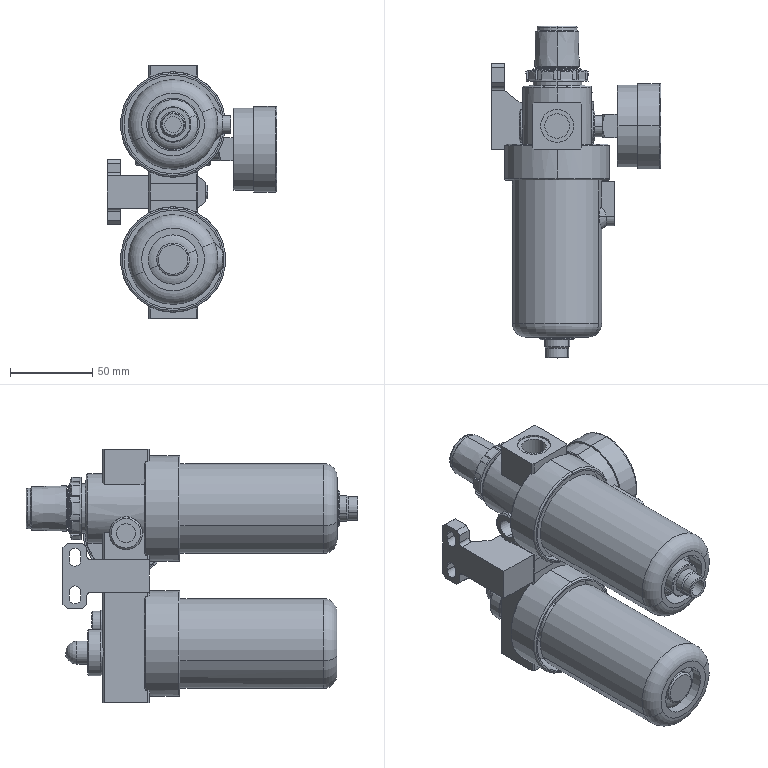Part | SolidWorks | 8 solids | 386 faces | box 103 x 201.6 x 154 mm | volume 428441 mm3 | plane 173 | cylinder 128 | cone 54 | torus 30 | sphere 1 | commonest cylinder face diameters 35.7 x11 20 x10 14.95 x8 19.994 x8 7 x6 6 x4